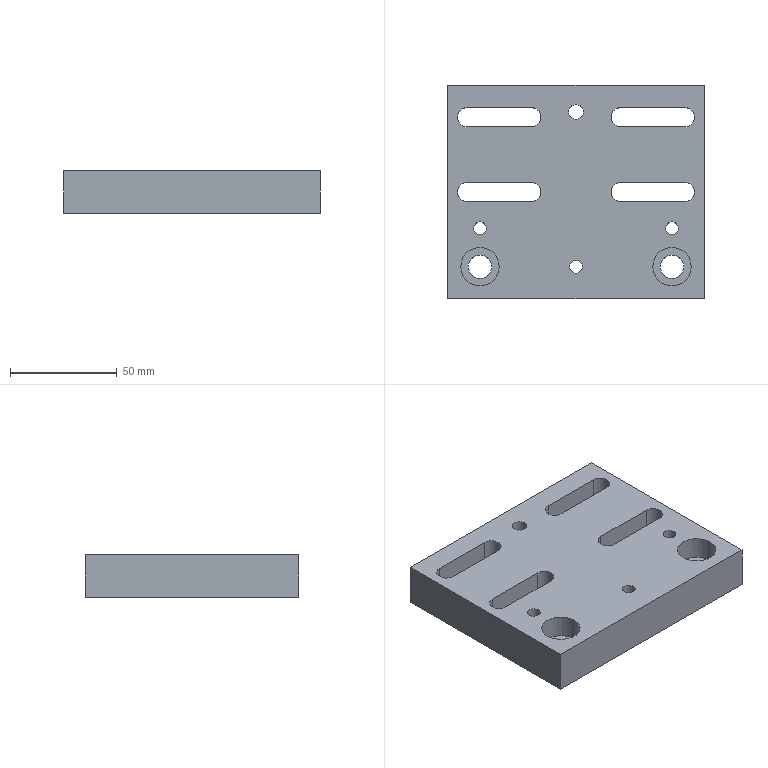Part | NX | 1 solid | 32 faces | box 120 x 100 x 20 mm | volume 203706 mm3 | plane 16 | cylinder 16 | commonest cylinder face diameters 9 x8 6 x3 11 x2 18 x2 6.8 x1
STEP:
#1=CARTESIAN_POINT('',(51.,89.5,0.));
#2=VERTEX_POINT('',#1);
#3=CARTESIAN_POINT('',(51.,89.5,20.));
#4=VERTEX_POINT('',#3);
#5=CARTESIAN_POINT('',(51.,89.5,0.));
#6=DIRECTION('',(0.,0.,1.));
#7=VECTOR('',#6,1000.);
#8=LINE('',#5,#7);
#9=EDGE_CURVE('',#2,#4,#8,.T.);
#10=ORIENTED_EDGE('',*,*,#9,.T.);
#11=CARTESIAN_POINT('',(21.,89.5,20.));
#12=VERTEX_POINT('',#11);
#13=CARTESIAN_POINT('',(21.,89.5,20.));
#14=DIRECTION('',(1.,0.,0.));
#15=VECTOR('',#14,1000.);
#16=LINE('',#13,#15);
#17=EDGE_CURVE('',#12,#4,#16,.T.);
#18=ORIENTED_EDGE('',*,*,#17,.F.);
#19=CARTESIAN_POINT('',(21.,89.5,0.));
#20=VERTEX_POINT('',#19);
#21=CARTESIAN_POINT('',(21.,89.5,0.));
#22=DIRECTION('',(0.,0.,-1.));
#23=VECTOR('',#22,1000.);
#24=LINE('',#21,#23);
#25=EDGE_CURVE('',#12,#20,#24,.T.);
#26=ORIENTED_EDGE('',*,*,#25,.T.);
#27=CARTESIAN_POINT('',(21.,89.5,0.));
#28=DIRECTION('',(1.,0.,0.));
#29=VECTOR('',#28,1000.);
#30=LINE('',#27,#29);
#31=EDGE_CURVE('',#20,#2,#30,.T.);
#32=ORIENTED_EDGE('',*,*,#31,.T.);
#33=EDGE_LOOP('',(#10,#18,#26,#32));
#34=FACE_BOUND('',#33,.T.);
#35=CARTESIAN_POINT('',(21.,89.5,0.));
#36=DIRECTION('',(0.,1.,0.));
#37=DIRECTION('',(0.,0.,1.));
#38=AXIS2_PLACEMENT_3D('',#35,#36,#37);
#39=PLANE('',#38);
#40=ADVANCED_FACE('',(#34),#39,.F.);
#41=CARTESIAN_POINT('',(51.,80.5,20.));
#42=VERTEX_POINT('',#41);
#43=CARTESIAN_POINT('',(51.,80.5,0.));
#44=VERTEX_POINT('',#43);
#45=CARTESIAN_POINT('',(51.,80.5,0.));
#46=DIRECTION('',(0.,0.,-1.));
#47=VECTOR('',#46,1000.);
#48=LINE('',#45,#47);
#49=EDGE_CURVE('',#42,#44,#48,.T.);
#50=ORIENTED_EDGE('',*,*,#49,.T.);
#51=CARTESIAN_POINT('',(21.,80.5,0.));
#52=VERTEX_POINT('',#51);
#53=CARTESIAN_POINT('',(21.,80.5,0.));
#54=DIRECTION('',(1.,0.,0.));
#55=VECTOR('',#54,1000.);
#56=LINE('',#53,#55);
#57=EDGE_CURVE('',#52,#44,#56,.T.);
#58=ORIENTED_EDGE('',*,*,#57,.F.);
#59=CARTESIAN_POINT('',(21.,80.5,20.));
#60=VERTEX_POINT('',#59);
#61=CARTESIAN_POINT('',(21.,80.5,0.));
#62=DIRECTION('',(0.,0.,1.));
#63=VECTOR('',#62,1000.);
#64=LINE('',#61,#63);
#65=EDGE_CURVE('',#52,#60,#64,.T.);
#66=ORIENTED_EDGE('',*,*,#65,.T.);
#67=CARTESIAN_POINT('',(21.,80.5,20.));
#68=DIRECTION('',(1.,0.,0.));
#69=VECTOR('',#68,1000.);
#70=LINE('',#67,#69);
#71=EDGE_CURVE('',#60,#42,#70,.T.);
#72=ORIENTED_EDGE('',*,*,#71,.T.);
#73=EDGE_LOOP('',(#50,#58,#66,#72));
#74=FACE_BOUND('',#73,.T.);
#75=CARTESIAN_POINT('',(21.,80.5,0.));
#76=DIRECTION('',(0.,-1.,0.));
#77=DIRECTION('',(0.,0.,-1.));
#78=AXIS2_PLACEMENT_3D('',#75,#76,#77);
#79=PLANE('',#78);
#80=ADVANCED_FACE('',(#74),#79,.F.);
#81=CARTESIAN_POINT('',(51.,85.,20.));
#82=DIRECTION('',(0.,0.,-1.));
#83=DIRECTION('',(-1.,0.,0.));
#84=AXIS2_PLACEMENT_3D('',#81,#82,#83);
#85=CIRCLE('',#84,4.5);
#86=EDGE_CURVE('',#4,#42,#85,.T.);
#87=ORIENTED_EDGE('',*,*,#86,.F.);
#88=ORIENTED_EDGE('',*,*,#9,.F.);
#89=CARTESIAN_POINT('',(51.,85.,0.));
#90=DIRECTION('',(0.,0.,-1.));
#91=DIRECTION('',(-1.,0.,0.));
#92=AXIS2_PLACEMENT_3D('',#89,#90,#91);
#93=CIRCLE('',#92,4.5);
#94=EDGE_CURVE('',#2,#44,#93,.T.);
#95=ORIENTED_EDGE('',*,*,#94,.T.);
#96=ORIENTED_EDGE('',*,*,#49,.F.);
#97=EDGE_LOOP('',(#87,#88,#95,#96));
#98=FACE_BOUND('',#97,.T.);
#99=CARTESIAN_POINT('',(51.,85.,0.));
#100=DIRECTION('',(0.,0.,-1.));
#101=DIRECTION('',(-1.,0.,0.));
#102=AXIS2_PLACEMENT_3D('',#99,#100,#101);
#103=CYLINDRICAL_SURFACE('',#102,4.5);
#104=ADVANCED_FACE('',(#98),#103,.F.);
#105=CARTESIAN_POINT('',(51.,54.5,0.));
#106=VERTEX_POINT('',#105);
#107=CARTESIAN_POINT('',(51.,54.5,20.));
#108=VERTEX_POINT('',#107);
#109=CARTESIAN_POINT('',(51.,54.5,0.));
#110=DIRECTION('',(0.,0.,1.));
#111=VECTOR('',#110,1000.);
#112=LINE('',#109,#111);
#113=EDGE_CURVE('',#106,#108,#112,.T.);
#114=ORIENTED_EDGE('',*,*,#113,.T.);
#115=CARTESIAN_POINT('',(21.,54.5,20.));
#116=VERTEX_POINT('',#115);
#117=CARTESIAN_POINT('',(21.,54.5,20.));
#118=DIRECTION('',(1.,0.,0.));
#119=VECTOR('',#118,1000.);
#120=LINE('',#117,#119);
#121=EDGE_CURVE('',#116,#108,#120,.T.);
#122=ORIENTED_EDGE('',*,*,#121,.F.);
#123=CARTESIAN_POINT('',(21.,54.5,0.));
#124=VERTEX_POINT('',#123);
#125=CARTESIAN_POINT('',(21.,54.5,0.));
#126=DIRECTION('',(0.,0.,-1.));
#127=VECTOR('',#126,1000.);
#128=LINE('',#125,#127);
#129=EDGE_CURVE('',#116,#124,#128,.T.);
#130=ORIENTED_EDGE('',*,*,#129,.T.);
#131=CARTESIAN_POINT('',(21.,54.5,0.));
#132=DIRECTION('',(1.,0.,0.));
#133=VECTOR('',#132,1000.);
#134=LINE('',#131,#133);
#135=EDGE_CURVE('',#124,#106,#134,.T.);
#136=ORIENTED_EDGE('',*,*,#135,.T.);
#137=EDGE_LOOP('',(#114,#122,#130,#136));
#138=FACE_BOUND('',#137,.T.);
#139=CARTESIAN_POINT('',(21.,54.5,0.));
#140=DIRECTION('',(0.,1.,0.));
#141=DIRECTION('',(0.,0.,1.));
#142=AXIS2_PLACEMENT_3D('',#139,#140,#141);
#143=PLANE('',#142);
#144=ADVANCED_FACE('',(#138),#143,.F.);
#145=CARTESIAN_POINT('',(51.,45.5,20.));
#146=VERTEX_POINT('',#145);
#147=CARTESIAN_POINT('',(51.,45.5,0.));
#148=VERTEX_POINT('',#147);
#149=CARTESIAN_POINT('',(51.,45.5,0.));
#150=DIRECTION('',(0.,0.,-1.));
#151=VECTOR('',#150,1000.);
#152=LINE('',#149,#151);
#153=EDGE_CURVE('',#146,#148,#152,.T.);
#154=ORIENTED_EDGE('',*,*,#153,.T.);
#155=CARTESIAN_POINT('',(21.,45.5,0.));
#156=VERTEX_POINT('',#155);
#157=CARTESIAN_POINT('',(21.,45.5,0.));
#158=DIRECTION('',(1.,0.,0.));
#159=VECTOR('',#158,1000.);
#160=LINE('',#157,#159);
#161=EDGE_CURVE('',#156,#148,#160,.T.);
#162=ORIENTED_EDGE('',*,*,#161,.F.);
#163=CARTESIAN_POINT('',(21.,45.5,20.));
#164=VERTEX_POINT('',#163);
#165=CARTESIAN_POINT('',(21.,45.5,0.));
#166=DIRECTION('',(0.,0.,1.));
#167=VECTOR('',#166,1000.);
#168=LINE('',#165,#167);
#169=EDGE_CURVE('',#156,#164,#168,.T.);
#170=ORIENTED_EDGE('',*,*,#169,.T.);
#171=CARTESIAN_POINT('',(21.,45.5,20.));
#172=DIRECTION('',(1.,0.,0.));
#173=VECTOR('',#172,1000.);
#174=LINE('',#171,#173);
#175=EDGE_CURVE('',#164,#146,#174,.T.);
#176=ORIENTED_EDGE('',*,*,#175,.T.);
#177=EDGE_LOOP('',(#154,#162,#170,#176));
#178=FACE_BOUND('',#177,.T.);
#179=CARTESIAN_POINT('',(21.,45.5,0.));
#180=DIRECTION('',(0.,-1.,0.));
#181=DIRECTION('',(0.,0.,-1.));
#182=AXIS2_PLACEMENT_3D('',#179,#180,#181);
#183=PLANE('',#182);
#184=ADVANCED_FACE('',(#178),#183,.F.);
#185=CARTESIAN_POINT('',(51.,50.,20.));
#186=DIRECTION('',(0.,0.,-1.));
#187=DIRECTION('',(-1.,0.,0.));
#188=AXIS2_PLACEMENT_3D('',#185,#186,#187);
#189=CIRCLE('',#188,4.5);
#190=EDGE_CURVE('',#108,#146,#189,.T.);
#191=ORIENTED_EDGE('',*,*,#190,.F.);
#192=ORIENTED_EDGE('',*,*,#113,.F.);
#193=CARTESIAN_POINT('',(51.,50.,0.));
#194=DIRECTION('',(0.,0.,-1.));
#195=DIRECTION('',(-1.,0.,0.));
#196=AXIS2_PLACEMENT_3D('',#193,#194,#195);
#197=CIRCLE('',#196,4.5);
#198=EDGE_CURVE('',#106,#148,#197,.T.);
#199=ORIENTED_EDGE('',*,*,#198,.T.);
#200=ORIENTED_EDGE('',*,*,#153,.F.);
#201=EDGE_LOOP('',(#191,#192,#199,#200));
#202=FACE_BOUND('',#201,.T.);
#203=CARTESIAN_POINT('',(51.,50.,0.));
#204=DIRECTION('',(0.,0.,-1.));
#205=DIRECTION('',(-1.,0.,0.));
#206=AXIS2_PLACEMENT_3D('',#203,#204,#205);
#207=CYLINDRICAL_SURFACE('',#206,4.5);
#208=ADVANCED_FACE('',(#202),#207,.F.);
#209=CARTESIAN_POINT('',(-21.,89.5,0.));
#210=VERTEX_POINT('',#209);
#211=CARTESIAN_POINT('',(-21.,89.5,20.));
#212=VERTEX_POINT('',#211);
#213=CARTESIAN_POINT('',(-21.,89.5,0.));
#214=DIRECTION('',(0.,0.,1.));
#215=VECTOR('',#214,1000.);
#216=LINE('',#213,#215);
#217=EDGE_CURVE('',#210,#212,#216,.T.);
#218=ORIENTED_EDGE('',*,*,#217,.T.);
#219=CARTESIAN_POINT('',(-51.,89.5,20.));
#220=VERTEX_POINT('',#219);
#221=CARTESIAN_POINT('',(0.,89.5,20.));
#222=DIRECTION('',(1.,0.,0.));
#223=VECTOR('',#222,1000.);
#224=LINE('',#221,#223);
#225=EDGE_CURVE('',#220,#212,#224,.T.);
#226=ORIENTED_EDGE('',*,*,#225,.F.);
#227=CARTESIAN_POINT('',(-51.,89.5,0.));
#228=VERTEX_POINT('',#227);
#229=CARTESIAN_POINT('',(-51.,89.5,0.));
#230=DIRECTION('',(0.,0.,-1.));
#231=VECTOR('',#230,1000.);
#232=LINE('',#229,#231);
#233=EDGE_CURVE('',#220,#228,#232,.T.);
#234=ORIENTED_EDGE('',*,*,#233,.T.);
#235=CARTESIAN_POINT('',(21.,89.5,0.));
#236=DIRECTION('',(1.,0.,0.));
#237=VECTOR('',#236,1000.);
#238=LINE('',#235,#237);
#239=EDGE_CURVE('',#228,#210,#238,.T.);
#240=ORIENTED_EDGE('',*,*,#239,.T.);
#241=EDGE_LOOP('',(#218,#226,#234,#240));
#242=FACE_BOUND('',#241,.T.);
#243=CARTESIAN_POINT('',(21.,89.5,0.));
#244=DIRECTION('',(0.,1.,0.));
#245=DIRECTION('',(0.,0.,1.));
#246=AXIS2_PLACEMENT_3D('',#243,#244,#245);
#247=PLANE('',#246);
#248=ADVANCED_FACE('',(#242),#247,.F.);
#249=CARTESIAN_POINT('',(-21.,80.5,20.));
#250=VERTEX_POINT('',#249);
#251=CARTESIAN_POINT('',(-21.,80.5,0.));
#252=VERTEX_POINT('',#251);
#253=CARTESIAN_POINT('',(-21.,80.5,0.));
#254=DIRECTION('',(0.,0.,-1.));
#255=VECTOR('',#254,1000.);
#256=LINE('',#253,#255);
#257=EDGE_CURVE('',#250,#252,#256,.T.);
#258=ORIENTED_EDGE('',*,*,#257,.T.);
#259=CARTESIAN_POINT('',(-51.,80.5,0.));
#260=VERTEX_POINT('',#259);
#261=CARTESIAN_POINT('',(0.,80.5,0.));
#262=DIRECTION('',(1.,0.,0.));
#263=VECTOR('',#262,1000.);
#264=LINE('',#261,#263);
#265=EDGE_CURVE('',#260,#252,#264,.T.);
#266=ORIENTED_EDGE('',*,*,#265,.F.);
#267=CARTESIAN_POINT('',(-51.,80.5,20.));
#268=VERTEX_POINT('',#267);
#269=CARTESIAN_POINT('',(-51.,80.5,0.));
#270=DIRECTION('',(0.,0.,1.));
#271=VECTOR('',#270,1000.);
#272=LINE('',#269,#271);
#273=EDGE_CURVE('',#260,#268,#272,.T.);
#274=ORIENTED_EDGE('',*,*,#273,.T.);
#275=CARTESIAN_POINT('',(21.,80.5,20.));
#276=DIRECTION('',(1.,0.,0.));
#277=VECTOR('',#276,1000.);
#278=LINE('',#275,#277);
#279=EDGE_CURVE('',#268,#250,#278,.T.);
#280=ORIENTED_EDGE('',*,*,#279,.T.);
#281=EDGE_LOOP('',(#258,#266,#274,#280));
#282=FACE_BOUND('',#281,.T.);
#283=CARTESIAN_POINT('',(21.,80.5,0.));
#284=DIRECTION('',(0.,-1.,0.));
#285=DIRECTION('',(0.,0.,-1.));
#286=AXIS2_PLACEMENT_3D('',#283,#284,#285);
#287=PLANE('',#286);
#288=ADVANCED_FACE('',(#282),#287,.F.);
#289=CARTESIAN_POINT('',(-21.,85.,20.));
#290=DIRECTION('',(0.,0.,-1.));
#291=DIRECTION('',(-1.,0.,0.));
#292=AXIS2_PLACEMENT_3D('',#289,#290,#291);
#293=CIRCLE('',#292,4.5);
#294=EDGE_CURVE('',#212,#250,#293,.T.);
#295=ORIENTED_EDGE('',*,*,#294,.F.);
#296=ORIENTED_EDGE('',*,*,#217,.F.);
#297=CARTESIAN_POINT('',(-21.,85.,0.));
#298=DIRECTION('',(0.,0.,-1.));
#299=DIRECTION('',(-1.,0.,0.));
#300=AXIS2_PLACEMENT_3D('',#297,#298,#299);
#301=CIRCLE('',#300,4.5);
#302=EDGE_CURVE('',#210,#252,#301,.T.);
#303=ORIENTED_EDGE('',*,*,#302,.T.);
#304=ORIENTED_EDGE('',*,*,#257,.F.);
#305=EDGE_LOOP('',(#295,#296,#303,#304));
#306=FACE_BOUND('',#305,.T.);
#307=CARTESIAN_POINT('',(-21.,85.,0.));
#308=DIRECTION('',(0.,0.,-1.));
#309=DIRECTION('',(-1.,0.,0.));
#310=AXIS2_PLACEMENT_3D('',#307,#308,#309);
#311=CYLINDRICAL_SURFACE('',#310,4.5);
#312=ADVANCED_FACE('',(#306),#311,.F.);
#313=CARTESIAN_POINT('',(-21.,54.5,0.));
#314=VERTEX_POINT('',#313);
#315=CARTESIAN_POINT('',(-21.,54.5,20.));
#316=VERTEX_POINT('',#315);
#317=CARTESIAN_POINT('',(-21.,54.5,0.));
#318=DIRECTION('',(0.,0.,1.));
#319=VECTOR('',#318,1000.);
#320=LINE('',#317,#319);
#321=EDGE_CURVE('',#314,#316,#320,.T.);
#322=ORIENTED_EDGE('',*,*,#321,.T.);
#323=CARTESIAN_POINT('',(-51.,54.5,20.));
#324=VERTEX_POINT('',#323);
#325=CARTESIAN_POINT('',(0.,54.5,20.));
#326=DIRECTION('',(1.,0.,0.));
#327=VECTOR('',#326,1000.);
#328=LINE('',#325,#327);
#329=EDGE_CURVE('',#324,#316,#328,.T.);
#330=ORIENTED_EDGE('',*,*,#329,.F.);
#331=CARTESIAN_POINT('',(-51.,54.5,0.));
#332=VERTEX_POINT('',#331);
#333=CARTESIAN_POINT('',(-51.,54.5,0.));
#334=DIRECTION('',(0.,0.,-1.));
#335=VECTOR('',#334,1000.);
#336=LINE('',#333,#335);
#337=EDGE_CURVE('',#324,#332,#336,.T.);
#338=ORIENTED_EDGE('',*,*,#337,.T.);
#339=CARTESIAN_POINT('',(21.,54.5,0.));
#340=DIRECTION('',(1.,0.,0.));
#341=VECTOR('',#340,1000.);
#342=LINE('',#339,#341);
#343=EDGE_CURVE('',#332,#314,#342,.T.);
#344=ORIENTED_EDGE('',*,*,#343,.T.);
#345=EDGE_LOOP('',(#322,#330,#338,#344));
#346=FACE_BOUND('',#345,.T.);
#347=CARTESIAN_POINT('',(21.,54.5,0.));
#348=DIRECTION('',(0.,1.,0.));
#349=DIRECTION('',(0.,0.,1.));
#350=AXIS2_PLACEMENT_3D('',#347,#348,#349);
#351=PLANE('',#350);
#352=ADVANCED_FACE('',(#346),#351,.F.);
#353=CARTESIAN_POINT('',(-21.,45.5,20.));
#354=VERTEX_POINT('',#353);
#355=CARTESIAN_POINT('',(-21.,45.5,0.));
#356=VERTEX_POINT('',#355);
#357=CARTESIAN_POINT('',(-21.,45.5,0.));
#358=DIRECTION('',(0.,0.,-1.));
#359=VECTOR('',#358,1000.);
#360=LINE('',#357,#359);
#361=EDGE_CURVE('',#354,#356,#360,.T.);
#362=ORIENTED_EDGE('',*,*,#361,.T.);
#363=CARTESIAN_POINT('',(-51.,45.5,0.));
#364=VERTEX_POINT('',#363);
#365=CARTESIAN_POINT('',(0.,45.5,0.));
#366=DIRECTION('',(1.,0.,0.));
#367=VECTOR('',#366,1000.);
#368=LINE('',#365,#367);
#369=EDGE_CURVE('',#364,#356,#368,.T.);
#370=ORIENTED_EDGE('',*,*,#369,.F.);
#371=CARTESIAN_POINT('',(-51.,45.5,20.));
#372=VERTEX_POINT('',#371);
#373=CARTESIAN_POINT('',(-51.,45.5,0.));
#374=DIRECTION('',(0.,0.,1.));
#375=VECTOR('',#374,1000.);
#376=LINE('',#373,#375);
#377=EDGE_CURVE('',#364,#372,#376,.T.);
#378=ORIENTED_EDGE('',*,*,#377,.T.);
#379=CARTESIAN_POINT('',(21.,45.5,20.));
#380=DIRECTION('',(1.,0.,0.));
#381=VECTOR('',#380,1000.);
#382=LINE('',#379,#381);
#383=EDGE_CURVE('',#372,#354,#382,.T.);
#384=ORIENTED_EDGE('',*,*,#383,.T.);
#385=EDGE_LOOP('',(#362,#370,#378,#384));
#386=FACE_BOUND('',#385,.T.);
#387=CARTESIAN_POINT('',(21.,45.5,0.));
#388=DIRECTION('',(0.,-1.,0.));
#389=DIRECTION('',(0.,0.,-1.));
#390=AXIS2_PLACEMENT_3D('',#387,#388,#389);
#391=PLANE('',#390);
#392=ADVANCED_FACE('',(#386),#391,.F.);
#393=CARTESIAN_POINT('',(-21.,50.,20.));
#394=DIRECTION('',(0.,0.,-1.));
#395=DIRECTION('',(-1.,0.,0.));
#396=AXIS2_PLACEMENT_3D('',#393,#394,#395);
#397=CIRCLE('',#396,4.5);
#398=EDGE_CURVE('',#316,#354,#397,.T.);
#399=ORIENTED_EDGE('',*,*,#398,.F.);
#400=ORIENTED_EDGE('',*,*,#321,.F.);
#401=CARTESIAN_POINT('',(-21.,50.,0.));
#402=DIRECTION('',(0.,0.,-1.));
#403=DIRECTION('',(-1.,0.,0.));
#404=AXIS2_PLACEMENT_3D('',#401,#402,#403);
#405=CIRCLE('',#404,4.5);
#406=EDGE_CURVE('',#314,#356,#405,.T.);
#407=ORIENTED_EDGE('',*,*,#406,.T.);
#408=ORIENTED_EDGE('',*,*,#361,.F.);
#409=EDGE_LOOP('',(#399,#400,#407,#408));
#410=FACE_BOUND('',#409,.T.);
#411=CARTESIAN_POINT('',(-21.,50.,0.));
#412=DIRECTION('',(0.,0.,-1.));
#413=DIRECTION('',(-1.,0.,0.));
#414=AXIS2_PLACEMENT_3D('',#411,#412,#413);
#415=CYLINDRICAL_SURFACE('',#414,4.5);
#416=ADVANCED_FACE('',(#410),#415,.F.);
#417=CARTESIAN_POINT('',(54.,15.,9.4));
#418=VERTEX_POINT('',#417);
#419=CARTESIAN_POINT('',(45.,15.,9.4));
#420=DIRECTION('',(0.,0.,1.));
#421=DIRECTION('',(1.,0.,0.));
#422=AXIS2_PLACEMENT_3D('',#419,#420,#421);
#423=CIRCLE('',#422,9.);
#424=EDGE_CURVE('',#418,#418,#423,.T.);
#425=ORIENTED_EDGE('',*,*,#424,.T.);
#426=EDGE_LOOP('',(#425));
#427=FACE_BOUND('',#426,.T.);
#428=CARTESIAN_POINT('',(50.5,15.,9.4));
#429=VERTEX_POINT('',#428);
#430=CARTESIAN_POINT('',(45.,15.,9.4));
#431=DIRECTION('',(0.,0.,1.));
#432=DIRECTION('',(1.,0.,0.));
#433=AXIS2_PLACEMENT_3D('',#430,#431,#432);
#434=CIRCLE('',#433,5.5);
#435=EDGE_CURVE('',#429,#429,#434,.T.);
#436=ORIENTED_EDGE('',*,*,#435,.F.);
#437=EDGE_LOOP('',(#436));
#438=FACE_BOUND('',#437,.T.);
#439=CARTESIAN_POINT('',(50.5,15.,9.4));
#440=DIRECTION('',(0.,0.,-1.));
#441=DIRECTION('',(-1.,0.,0.));
#442=AXIS2_PLACEMENT_3D('',#439,#440,#441);
#443=PLANE('',#442);
#444=ADVANCED_FACE('',(#427,#438),#443,.F.);
#445=CARTESIAN_POINT('',(-54.,15.,9.4));
#446=VERTEX_POINT('',#445);
#447=CARTESIAN_POINT('',(-45.,15.,9.4));
#448=DIRECTION('',(0.,0.,1.));
#449=DIRECTION('',(-1.,0.,0.));
#450=AXIS2_PLACEMENT_3D('',#447,#448,#449);
#451=CIRCLE('',#450,9.);
#452=EDGE_CURVE('',#446,#446,#451,.T.);
#453=ORIENTED_EDGE('',*,*,#452,.T.);
#454=EDGE_LOOP('',(#453));
#455=FACE_BOUND('',#454,.T.);
#456=CARTESIAN_POINT('',(-50.5,15.,9.4));
#457=VERTEX_POINT('',#456);
#458=CARTESIAN_POINT('',(-45.,15.,9.4));
#459=DIRECTION('',(0.,0.,1.));
#460=DIRECTION('',(-1.,0.,0.));
#461=AXIS2_PLACEMENT_3D('',#458,#459,#460);
#462=CIRCLE('',#461,5.5);
#463=EDGE_CURVE('',#457,#457,#462,.T.);
#464=ORIENTED_EDGE('',*,*,#463,.F.);
#465=EDGE_LOOP('',(#464));
#466=FACE_BOUND('',#465,.T.);
#467=CARTESIAN_POINT('',(50.5,15.,9.4));
#468=DIRECTION('',(0.,0.,-1.));
#469=DIRECTION('',(-1.,0.,0.));
#470=AXIS2_PLACEMENT_3D('',#467,#468,#469);
#471=PLANE('',#470);
#472=ADVANCED_FACE('',(#455,#466),#471,.F.);
#473=CARTESIAN_POINT('',(-60.,100.,0.));
#474=VERTEX_POINT('',#473);
#475=CARTESIAN_POINT('',(-60.,0.,0.));
#476=VERTEX_POINT('',#475);
#477=CARTESIAN_POINT('',(-60.,0.,0.));
#478=DIRECTION('',(0.,-1.,0.));
#479=VECTOR('',#478,1000.);
#480=LINE('',#477,#479);
#481=EDGE_CURVE('',#474,#476,#480,.T.);
#482=ORIENTED_EDGE('',*,*,#481,.F.);
#483=CARTESIAN_POINT('',(60.,100.,0.));
#484=VERTEX_POINT('',#483);
#485=CARTESIAN_POINT('',(-60.,100.,0.));
#486=DIRECTION('',(-1.,0.,0.));
#487=VECTOR('',#486,1000.);
#488=LINE('',#485,#487);
#489=EDGE_CURVE('',#484,#474,#488,.T.);
#490=ORIENTED_EDGE('',*,*,#489,.F.);
#491=CARTESIAN_POINT('',(60.,0.,0.));
#492=VERTEX_POINT('',#491);
#493=CARTESIAN_POINT('',(60.,0.,0.));
#494=DIRECTION('',(0.,1.,0.));
#495=VECTOR('',#494,1000.);
#496=LINE('',#493,#495);
#497=EDGE_CURVE('',#492,#484,#496,.T.);
#498=ORIENTED_EDGE('',*,*,#497,.F.);
#499=CARTESIAN_POINT('',(-60.,0.,0.));
#500=DIRECTION('',(1.,0.,0.));
#501=VECTOR('',#500,1000.);
#502=LINE('',#499,#501);
#503=EDGE_CURVE('',#476,#492,#502,.T.);
#504=ORIENTED_EDGE('',*,*,#503,.F.);
#505=EDGE_LOOP('',(#482,#490,#498,#504));
#506=FACE_BOUND('',#505,.T.);
#507=CARTESIAN_POINT('',(-39.5,15.,0.));
#508=VERTEX_POINT('',#507);
#509=CARTESIAN_POINT('',(-45.,15.,0.));
#510=DIRECTION('',(0.,0.,1.));
#511=DIRECTION('',(1.,0.,0.));
#512=AXIS2_PLACEMENT_3D('',#509,#510,#511);
#513=CIRCLE('',#512,5.5);
#514=EDGE_CURVE('',#508,#508,#513,.T.);
#515=ORIENTED_EDGE('',*,*,#514,.T.);
#516=EDGE_LOOP('',(#515));
#517=FACE_BOUND('',#516,.T.);
#518=CARTESIAN_POINT('',(50.5,15.,0.));
#519=VERTEX_POINT('',#518);
#520=CARTESIAN_POINT('',(45.,15.,0.));
#521=DIRECTION('',(0.,0.,1.));
#522=DIRECTION('',(1.,0.,0.));
#523=AXIS2_PLACEMENT_3D('',#520,#521,#522);
#524=CIRCLE('',#523,5.5);
#525=EDGE_CURVE('',#519,#519,#524,.T.);
#526=ORIENTED_EDGE('',*,*,#525,.T.);
#527=EDGE_LOOP('',(#526));
#528=FACE_BOUND('',#527,.T.);
#529=CARTESIAN_POINT('',(42.,33.,0.));
#530=VERTEX_POINT('',#529);
#531=CARTESIAN_POINT('',(45.,33.,0.));
#532=DIRECTION('',(0.,0.,-1.));
#533=DIRECTION('',(-1.,0.,0.));
#534=AXIS2_PLACEMENT_3D('',#531,#532,#533);
#535=CIRCLE('',#534,3.);
#536=EDGE_CURVE('',#530,#530,#535,.T.);
#537=ORIENTED_EDGE('',*,*,#536,.F.);
#538=EDGE_LOOP('',(#537));
#539=FACE_BOUND('',#538,.T.);
#540=CARTESIAN_POINT('',(-48.,33.,0.));
#541=VERTEX_POINT('',#540);
#542=CARTESIAN_POINT('',(-45.,33.,0.));
#543=DIRECTION('',(0.,0.,-1.));
#544=DIRECTION('',(-1.,0.,0.));
#545=AXIS2_PLACEMENT_3D('',#542,#543,#544);
#546=CIRCLE('',#545,3.);
#547=EDGE_CURVE('',#541,#541,#546,.T.);
#548=ORIENTED_EDGE('',*,*,#547,.F.);
#549=EDGE_LOOP('',(#548));
#550=FACE_BOUND('',#549,.T.);
#551=CARTESIAN_POINT('',(-3.,15.,0.));
#552=VERTEX_POINT('',#551);
#553=CARTESIAN_POINT('',(0.,15.,0.));
#554=DIRECTION('',(0.,0.,-1.));
#555=DIRECTION('',(-1.,0.,0.));
#556=AXIS2_PLACEMENT_3D('',#553,#554,#555);
#557=CIRCLE('',#556,3.);
#558=EDGE_CURVE('',#552,#552,#557,.T.);
#559=ORIENTED_EDGE('',*,*,#558,.F.);
#560=EDGE_LOOP('',(#559));
#561=FACE_BOUND('',#560,.T.);
#562=ORIENTED_EDGE('',*,*,#406,.F.);
#563=ORIENTED_EDGE('',*,*,#343,.F.);
#564=CARTESIAN_POINT('',(-51.,50.,0.));
#565=DIRECTION('',(0.,0.,-1.));
#566=DIRECTION('',(-1.,0.,0.));
#567=AXIS2_PLACEMENT_3D('',#564,#565,#566);
#568=CIRCLE('',#567,4.5);
#569=EDGE_CURVE('',#364,#332,#568,.T.);
#570=ORIENTED_EDGE('',*,*,#569,.F.);
#571=ORIENTED_EDGE('',*,*,#369,.T.);
#572=EDGE_LOOP('',(#562,#563,#570,#571));
#573=FACE_BOUND('',#572,.T.);
#574=ORIENTED_EDGE('',*,*,#302,.F.);
#575=ORIENTED_EDGE('',*,*,#239,.F.);
#576=CARTESIAN_POINT('',(-51.,85.,0.));
#577=DIRECTION('',(0.,0.,-1.));
#578=DIRECTION('',(-1.,0.,0.));
#579=AXIS2_PLACEMENT_3D('',#576,#577,#578);
#580=CIRCLE('',#579,4.5);
#581=EDGE_CURVE('',#260,#228,#580,.T.);
#582=ORIENTED_EDGE('',*,*,#581,.F.);
#583=ORIENTED_EDGE('',*,*,#265,.T.);
#584=EDGE_LOOP('',(#574,#575,#582,#583));
#585=FACE_BOUND('',#584,.T.);
#586=ORIENTED_EDGE('',*,*,#198,.F.);
#587=ORIENTED_EDGE('',*,*,#135,.F.);
#588=CARTESIAN_POINT('',(21.,50.,0.));
#589=DIRECTION('',(0.,0.,-1.));
#590=DIRECTION('',(-1.,0.,0.));
#591=AXIS2_PLACEMENT_3D('',#588,#589,#590);
#592=CIRCLE('',#591,4.5);
#593=EDGE_CURVE('',#156,#124,#592,.T.);
#594=ORIENTED_EDGE('',*,*,#593,.F.);
#595=ORIENTED_EDGE('',*,*,#161,.T.);
#596=EDGE_LOOP('',(#586,#587,#594,#595));
#597=FACE_BOUND('',#596,.T.);
#598=ORIENTED_EDGE('',*,*,#57,.T.);
#599=ORIENTED_EDGE('',*,*,#94,.F.);
#600=ORIENTED_EDGE('',*,*,#31,.F.);
#601=CARTESIAN_POINT('',(21.,85.,0.));
#602=DIRECTION('',(0.,0.,-1.));
#603=DIRECTION('',(-1.,0.,0.));
#604=AXIS2_PLACEMENT_3D('',#601,#602,#603);
#605=CIRCLE('',#604,4.5);
#606=EDGE_CURVE('',#52,#20,#605,.T.);
#607=ORIENTED_EDGE('',*,*,#606,.F.);
#608=EDGE_LOOP('',(#598,#599,#600,#607));
#609=FACE_BOUND('',#608,.T.);
#610=CARTESIAN_POINT('',(-3.4,87.5,0.));
#611=VERTEX_POINT('',#610);
#612=CARTESIAN_POINT('',(0.,87.5,0.));
#613=DIRECTION('',(0.,0.,-1.));
#614=DIRECTION('',(-1.,0.,0.));
#615=AXIS2_PLACEMENT_3D('',#612,#613,#614);
#616=CIRCLE('',#615,3.4);
#617=EDGE_CURVE('',#611,#611,#616,.T.);
#618=ORIENTED_EDGE('',*,*,#617,.F.);
#619=EDGE_LOOP('',(#618));
#620=FACE_BOUND('',#619,.T.);
#621=CARTESIAN_POINT('',(0.,0.,0.));
#622=DIRECTION('',(0.,0.,-1.));
#623=DIRECTION('',(-1.,0.,0.));
#624=AXIS2_PLACEMENT_3D('',#621,#622,#623);
#625=PLANE('',#624);
#626=ADVANCED_FACE('',(#506,#517,#528,#539,#550,#561,#573,#585,#597,#609,#620),#625,.T.);
#627=ORIENTED_EDGE('',*,*,#489,.T.);
#628=CARTESIAN_POINT('',(-60.,100.,20.));
#629=VERTEX_POINT('',#628);
#630=CARTESIAN_POINT('',(-60.,100.,20.));
#631=DIRECTION('',(0.,0.,-1.));
#632=VECTOR('',#631,1000.);
#633=LINE('',#630,#632);
#634=EDGE_CURVE('',#629,#474,#633,.T.);
#635=ORIENTED_EDGE('',*,*,#634,.F.);
#636=CARTESIAN_POINT('',(60.,100.,20.));
#637=VERTEX_POINT('',#636);
#638=CARTESIAN_POINT('',(-60.,100.,20.));
#639=DIRECTION('',(-1.,0.,0.));
#640=VECTOR('',#639,1000.);
#641=LINE('',#638,#640);
#642=EDGE_CURVE('',#637,#629,#641,.T.);
#643=ORIENTED_EDGE('',*,*,#642,.F.);
#644=CARTESIAN_POINT('',(60.,100.,20.));
#645=DIRECTION('',(0.,0.,-1.));
#646=VECTOR('',#645,1000.);
#647=LINE('',#644,#646);
#648=EDGE_CURVE('',#637,#484,#647,.T.);
#649=ORIENTED_EDGE('',*,*,#648,.T.);
#650=EDGE_LOOP('',(#627,#635,#643,#649));
#651=FACE_BOUND('',#650,.T.);
#652=CARTESIAN_POINT('',(-60.,100.,20.));
#653=DIRECTION('',(0.,-1.,0.));
#654=DIRECTION('',(0.,0.,-1.));
#655=AXIS2_PLACEMENT_3D('',#652,#653,#654);
#656=PLANE('',#655);
#657=ADVANCED_FACE('',(#651),#656,.F.);
#658=ORIENTED_EDGE('',*,*,#497,.T.);
#659=ORIENTED_EDGE('',*,*,#648,.F.);
#660=CARTESIAN_POINT('',(60.,0.,20.));
#661=VERTEX_POINT('',#660);
#662=CARTESIAN_POINT('',(60.,0.,20.));
#663=DIRECTION('',(0.,1.,0.));
#664=VECTOR('',#663,1000.);
#665=LINE('',#662,#664);
#666=EDGE_CURVE('',#661,#637,#665,.T.);
#667=ORIENTED_EDGE('',*,*,#666,.F.);
#668=CARTESIAN_POINT('',(60.,0.,20.));
#669=DIRECTION('',(0.,0.,-1.));
#670=VECTOR('',#669,1000.);
#671=LINE('',#668,#670);
#672=EDGE_CURVE('',#661,#492,#671,.T.);
#673=ORIENTED_EDGE('',*,*,#672,.T.);
#674=EDGE_LOOP('',(#658,#659,#667,#673));
#675=FACE_BOUND('',#674,.T.);
#676=CARTESIAN_POINT('',(60.,0.,20.));
#677=DIRECTION('',(-1.,0.,0.));
#678=DIRECTION('',(0.,0.,1.));
#679=AXIS2_PLACEMENT_3D('',#676,#677,#678);
#680=PLANE('',#679);
#681=ADVANCED_FACE('',(#675),#680,.F.);
#682=ORIENTED_EDGE('',*,*,#503,.T.);
#683=ORIENTED_EDGE('',*,*,#672,.F.);
#684=CARTESIAN_POINT('',(-60.,0.,20.));
#685=VERTEX_POINT('',#684);
#686=CARTESIAN_POINT('',(-60.,0.,20.));
#687=DIRECTION('',(1.,0.,0.));
#688=VECTOR('',#687,1000.);
#689=LINE('',#686,#688);
#690=EDGE_CURVE('',#685,#661,#689,.T.);
#691=ORIENTED_EDGE('',*,*,#690,.F.);
#692=CARTESIAN_POINT('',(-60.,0.,20.));
#693=DIRECTION('',(0.,0.,-1.));
#694=VECTOR('',#693,1000.);
#695=LINE('',#692,#694);
#696=EDGE_CURVE('',#685,#476,#695,.T.);
#697=ORIENTED_EDGE('',*,*,#696,.T.);
#698=EDGE_LOOP('',(#682,#683,#691,#697));
#699=FACE_BOUND('',#698,.T.);
#700=CARTESIAN_POINT('',(-60.,0.,20.));
#701=DIRECTION('',(0.,1.,0.));
#702=DIRECTION('',(0.,0.,1.));
#703=AXIS2_PLACEMENT_3D('',#700,#701,#702);
#704=PLANE('',#703);
#705=ADVANCED_FACE('',(#699),#704,.F.);
#706=ORIENTED_EDGE('',*,*,#481,.T.);
#707=ORIENTED_EDGE('',*,*,#696,.F.);
#708=CARTESIAN_POINT('',(-60.,0.,20.));
#709=DIRECTION('',(0.,-1.,0.));
#710=VECTOR('',#709,1000.);
#711=LINE('',#708,#710);
#712=EDGE_CURVE('',#629,#685,#711,.T.);
#713=ORIENTED_EDGE('',*,*,#712,.F.);
#714=ORIENTED_EDGE('',*,*,#634,.T.);
#715=EDGE_LOOP('',(#706,#707,#713,#714));
#716=FACE_BOUND('',#715,.T.);
#717=CARTESIAN_POINT('',(-60.,0.,20.));
#718=DIRECTION('',(1.,0.,0.));
#719=DIRECTION('',(0.,0.,-1.));
#720=AXIS2_PLACEMENT_3D('',#717,#718,#719);
#721=PLANE('',#720);
#722=ADVANCED_FACE('',(#716),#721,.F.);
#723=ORIENTED_EDGE('',*,*,#175,.F.);
#724=CARTESIAN_POINT('',(21.,50.,20.));
#725=DIRECTION('',(0.,0.,-1.));
#726=DIRECTION('',(-1.,0.,0.));
#727=AXIS2_PLACEMENT_3D('',#724,#725,#726);
#728=CIRCLE('',#727,4.5);
#729=EDGE_CURVE('',#164,#116,#728,.T.);
#730=ORIENTED_EDGE('',*,*,#729,.T.);
#731=ORIENTED_EDGE('',*,*,#121,.T.);
#732=ORIENTED_EDGE('',*,*,#190,.T.);
#733=EDGE_LOOP('',(#723,#730,#731,#732));
#734=FACE_BOUND('',#733,.T.);
#735=ORIENTED_EDGE('',*,*,#294,.T.);
#736=ORIENTED_EDGE('',*,*,#279,.F.);
#737=CARTESIAN_POINT('',(-51.,85.,20.));
#738=DIRECTION('',(0.,0.,-1.));
#739=DIRECTION('',(-1.,0.,0.));
#740=AXIS2_PLACEMENT_3D('',#737,#738,#739);
#741=CIRCLE('',#740,4.5);
#742=EDGE_CURVE('',#268,#220,#741,.T.);
#743=ORIENTED_EDGE('',*,*,#742,.T.);
#744=ORIENTED_EDGE('',*,*,#225,.T.);
#745=EDGE_LOOP('',(#735,#736,#743,#744));
#746=FACE_BOUND('',#745,.T.);
#747=ORIENTED_EDGE('',*,*,#329,.T.);
#748=ORIENTED_EDGE('',*,*,#398,.T.);
#749=ORIENTED_EDGE('',*,*,#383,.F.);
#750=CARTESIAN_POINT('',(-51.,50.,20.));
#751=DIRECTION('',(0.,0.,-1.));
#752=DIRECTION('',(-1.,0.,0.));
#753=AXIS2_PLACEMENT_3D('',#750,#751,#752);
#754=CIRCLE('',#753,4.5);
#755=EDGE_CURVE('',#372,#324,#754,.T.);
#756=ORIENTED_EDGE('',*,*,#755,.T.);
#757=EDGE_LOOP('',(#747,#748,#749,#756));
#758=FACE_BOUND('',#757,.T.);
#759=CARTESIAN_POINT('',(-3.,15.,20.));
#760=VERTEX_POINT('',#759);
#761=CARTESIAN_POINT('',(0.,15.,20.));
#762=DIRECTION('',(0.,0.,-1.));
#763=DIRECTION('',(-1.,0.,0.));
#764=AXIS2_PLACEMENT_3D('',#761,#762,#763);
#765=CIRCLE('',#764,3.);
#766=EDGE_CURVE('',#760,#760,#765,.T.);
#767=ORIENTED_EDGE('',*,*,#766,.T.);
#768=EDGE_LOOP('',(#767));
#769=FACE_BOUND('',#768,.T.);
#770=CARTESIAN_POINT('',(-48.,33.,20.));
#771=VERTEX_POINT('',#770);
#772=CARTESIAN_POINT('',(-45.,33.,20.));
#773=DIRECTION('',(0.,0.,-1.));
#774=DIRECTION('',(-1.,0.,0.));
#775=AXIS2_PLACEMENT_3D('',#772,#773,#774);
#776=CIRCLE('',#775,3.);
#777=EDGE_CURVE('',#771,#771,#776,.T.);
#778=ORIENTED_EDGE('',*,*,#777,.T.);
#779=EDGE_LOOP('',(#778));
#780=FACE_BOUND('',#779,.T.);
#781=CARTESIAN_POINT('',(42.,33.,20.));
#782=VERTEX_POINT('',#781);
#783=CARTESIAN_POINT('',(45.,33.,20.));
#784=DIRECTION('',(0.,0.,-1.));
#785=DIRECTION('',(-1.,0.,0.));
#786=AXIS2_PLACEMENT_3D('',#783,#784,#785);
#787=CIRCLE('',#786,3.);
#788=EDGE_CURVE('',#782,#782,#787,.T.);
#789=ORIENTED_EDGE('',*,*,#788,.T.);
#790=EDGE_LOOP('',(#789));
#791=FACE_BOUND('',#790,.T.);
#792=CARTESIAN_POINT('',(54.,15.,20.));
#793=VERTEX_POINT('',#792);
#794=CARTESIAN_POINT('',(45.,15.,20.));
#795=DIRECTION('',(0.,0.,1.));
#796=DIRECTION('',(1.,0.,0.));
#797=AXIS2_PLACEMENT_3D('',#794,#795,#796);
#798=CIRCLE('',#797,9.);
#799=EDGE_CURVE('',#793,#793,#798,.T.);
#800=ORIENTED_EDGE('',*,*,#799,.F.);
#801=EDGE_LOOP('',(#800));
#802=FACE_BOUND('',#801,.T.);
#803=CARTESIAN_POINT('',(-36.,15.,20.));
#804=VERTEX_POINT('',#803);
#805=CARTESIAN_POINT('',(-45.,15.,20.));
#806=DIRECTION('',(0.,0.,1.));
#807=DIRECTION('',(1.,0.,0.));
#808=AXIS2_PLACEMENT_3D('',#805,#806,#807);
#809=CIRCLE('',#808,9.);
#810=EDGE_CURVE('',#804,#804,#809,.T.);
#811=ORIENTED_EDGE('',*,*,#810,.F.);
#812=EDGE_LOOP('',(#811));
#813=FACE_BOUND('',#812,.T.);
#814=ORIENTED_EDGE('',*,*,#712,.T.);
#815=ORIENTED_EDGE('',*,*,#690,.T.);
#816=ORIENTED_EDGE('',*,*,#666,.T.);
#817=ORIENTED_EDGE('',*,*,#642,.T.);
#818=EDGE_LOOP('',(#814,#815,#816,#817));
#819=FACE_BOUND('',#818,.T.);
#820=ORIENTED_EDGE('',*,*,#17,.T.);
#821=ORIENTED_EDGE('',*,*,#86,.T.);
#822=ORIENTED_EDGE('',*,*,#71,.F.);
#823=CARTESIAN_POINT('',(21.,85.,20.));
#824=DIRECTION('',(0.,0.,-1.));
#825=DIRECTION('',(-1.,0.,0.));
#826=AXIS2_PLACEMENT_3D('',#823,#824,#825);
#827=CIRCLE('',#826,4.5);
#828=EDGE_CURVE('',#60,#12,#827,.T.);
#829=ORIENTED_EDGE('',*,*,#828,.T.);
#830=EDGE_LOOP('',(#820,#821,#822,#829));
#831=FACE_BOUND('',#830,.T.);
#832=CARTESIAN_POINT('',(-3.4,87.5,20.));
#833=VERTEX_POINT('',#832);
#834=CARTESIAN_POINT('',(0.,87.5,20.));
#835=DIRECTION('',(0.,0.,-1.));
#836=DIRECTION('',(-1.,0.,0.));
#837=AXIS2_PLACEMENT_3D('',#834,#835,#836);
#838=CIRCLE('',#837,3.4);
#839=EDGE_CURVE('',#833,#833,#838,.T.);
#840=ORIENTED_EDGE('',*,*,#839,.T.);
#841=EDGE_LOOP('',(#840));
#842=FACE_BOUND('',#841,.T.);
#843=CARTESIAN_POINT('',(0.,0.,20.));
#844=DIRECTION('',(0.,0.,-1.));
#845=DIRECTION('',(-1.,0.,0.));
#846=AXIS2_PLACEMENT_3D('',#843,#844,#845);
#847=PLANE('',#846);
#848=ADVANCED_FACE('',(#734,#746,#758,#769,#780,#791,#802,#813,#819,#831,#842),#847,.F.);
#849=ORIENTED_EDGE('',*,*,#514,.F.);
#850=EDGE_LOOP('',(#849));
#851=FACE_BOUND('',#850,.T.);
#852=ORIENTED_EDGE('',*,*,#463,.T.);
#853=EDGE_LOOP('',(#852));
#854=FACE_BOUND('',#853,.T.);
#855=CARTESIAN_POINT('',(-45.,15.,20.));
#856=DIRECTION('',(0.,0.,1.));
#857=DIRECTION('',(1.,0.,0.));
#858=AXIS2_PLACEMENT_3D('',#855,#856,#857);
#859=CYLINDRICAL_SURFACE('',#858,5.5);
#860=ADVANCED_FACE('',(#851,#854),#859,.F.);
#861=ORIENTED_EDGE('',*,*,#452,.F.);
#862=EDGE_LOOP('',(#861));
#863=FACE_BOUND('',#862,.T.);
#864=ORIENTED_EDGE('',*,*,#810,.T.);
#865=EDGE_LOOP('',(#864));
#866=FACE_BOUND('',#865,.T.);
#867=CARTESIAN_POINT('',(-45.,15.,20.));
#868=DIRECTION('',(0.,0.,1.));
#869=DIRECTION('',(1.,0.,0.));
#870=AXIS2_PLACEMENT_3D('',#867,#868,#869);
#871=CYLINDRICAL_SURFACE('',#870,9.);
#872=ADVANCED_FACE('',(#863,#866),#871,.F.);
#873=ORIENTED_EDGE('',*,*,#525,.F.);
#874=EDGE_LOOP('',(#873));
#875=FACE_BOUND('',#874,.T.);
#876=ORIENTED_EDGE('',*,*,#435,.T.);
#877=EDGE_LOOP('',(#876));
#878=FACE_BOUND('',#877,.T.);
#879=CARTESIAN_POINT('',(45.,15.,20.));
#880=DIRECTION('',(0.,0.,1.));
#881=DIRECTION('',(1.,0.,0.));
#882=AXIS2_PLACEMENT_3D('',#879,#880,#881);
#883=CYLINDRICAL_SURFACE('',#882,5.5);
#884=ADVANCED_FACE('',(#875,#878),#883,.F.);
#885=ORIENTED_EDGE('',*,*,#424,.F.);
#886=EDGE_LOOP('',(#885));
#887=FACE_BOUND('',#886,.T.);
#888=ORIENTED_EDGE('',*,*,#799,.T.);
#889=EDGE_LOOP('',(#888));
#890=FACE_BOUND('',#889,.T.);
#891=CARTESIAN_POINT('',(45.,15.,20.));
#892=DIRECTION('',(0.,0.,1.));
#893=DIRECTION('',(1.,0.,0.));
#894=AXIS2_PLACEMENT_3D('',#891,#892,#893);
#895=CYLINDRICAL_SURFACE('',#894,9.);
#896=ADVANCED_FACE('',(#887,#890),#895,.F.);
#897=ORIENTED_EDGE('',*,*,#536,.T.);
#898=EDGE_LOOP('',(#897));
#899=FACE_BOUND('',#898,.T.);
#900=ORIENTED_EDGE('',*,*,#788,.F.);
#901=EDGE_LOOP('',(#900));
#902=FACE_BOUND('',#901,.T.);
#903=CARTESIAN_POINT('',(45.,33.,0.));
#904=DIRECTION('',(0.,0.,-1.));
#905=DIRECTION('',(-1.,0.,0.));
#906=AXIS2_PLACEMENT_3D('',#903,#904,#905);
#907=CYLINDRICAL_SURFACE('',#906,3.);
#908=ADVANCED_FACE('',(#899,#902),#907,.F.);
#909=ORIENTED_EDGE('',*,*,#547,.T.);
#910=EDGE_LOOP('',(#909));
#911=FACE_BOUND('',#910,.T.);
#912=ORIENTED_EDGE('',*,*,#777,.F.);
#913=EDGE_LOOP('',(#912));
#914=FACE_BOUND('',#913,.T.);
#915=CARTESIAN_POINT('',(-45.,33.,0.));
#916=DIRECTION('',(0.,0.,-1.));
#917=DIRECTION('',(-1.,0.,0.));
#918=AXIS2_PLACEMENT_3D('',#915,#916,#917);
#919=CYLINDRICAL_SURFACE('',#918,3.);
#920=ADVANCED_FACE('',(#911,#914),#919,.F.);
#921=ORIENTED_EDGE('',*,*,#558,.T.);
#922=EDGE_LOOP('',(#921));
#923=FACE_BOUND('',#922,.T.);
#924=ORIENTED_EDGE('',*,*,#766,.F.);
#925=EDGE_LOOP('',(#924));
#926=FACE_BOUND('',#925,.T.);
#927=CARTESIAN_POINT('',(0.,15.,0.));
#928=DIRECTION('',(0.,0.,-1.));
#929=DIRECTION('',(-1.,0.,0.));
#930=AXIS2_PLACEMENT_3D('',#927,#928,#929);
#931=CYLINDRICAL_SURFACE('',#930,3.);
#932=ADVANCED_FACE('',(#923,#926),#931,.F.);
#933=ORIENTED_EDGE('',*,*,#755,.F.);
#934=ORIENTED_EDGE('',*,*,#377,.F.);
#935=ORIENTED_EDGE('',*,*,#569,.T.);
#936=ORIENTED_EDGE('',*,*,#337,.F.);
#937=EDGE_LOOP('',(#933,#934,#935,#936));
#938=FACE_BOUND('',#937,.T.);
#939=CARTESIAN_POINT('',(-51.,50.,0.));
#940=DIRECTION('',(0.,0.,-1.));
#941=DIRECTION('',(-1.,0.,0.));
#942=AXIS2_PLACEMENT_3D('',#939,#940,#941);
#943=CYLINDRICAL_SURFACE('',#942,4.5);
#944=ADVANCED_FACE('',(#938),#943,.F.);
#945=ORIENTED_EDGE('',*,*,#742,.F.);
#946=ORIENTED_EDGE('',*,*,#273,.F.);
#947=ORIENTED_EDGE('',*,*,#581,.T.);
#948=ORIENTED_EDGE('',*,*,#233,.F.);
#949=EDGE_LOOP('',(#945,#946,#947,#948));
#950=FACE_BOUND('',#949,.T.);
#951=CARTESIAN_POINT('',(-51.,85.,0.));
#952=DIRECTION('',(0.,0.,-1.));
#953=DIRECTION('',(-1.,0.,0.));
#954=AXIS2_PLACEMENT_3D('',#951,#952,#953);
#955=CYLINDRICAL_SURFACE('',#954,4.5);
#956=ADVANCED_FACE('',(#950),#955,.F.);
#957=ORIENTED_EDGE('',*,*,#729,.F.);
#958=ORIENTED_EDGE('',*,*,#169,.F.);
#959=ORIENTED_EDGE('',*,*,#593,.T.);
#960=ORIENTED_EDGE('',*,*,#129,.F.);
#961=EDGE_LOOP('',(#957,#958,#959,#960));
#962=FACE_BOUND('',#961,.T.);
#963=CARTESIAN_POINT('',(21.,50.,0.));
#964=DIRECTION('',(0.,0.,-1.));
#965=DIRECTION('',(-1.,0.,0.));
#966=AXIS2_PLACEMENT_3D('',#963,#964,#965);
#967=CYLINDRICAL_SURFACE('',#966,4.5);
#968=ADVANCED_FACE('',(#962),#967,.F.);
#969=ORIENTED_EDGE('',*,*,#828,.F.);
#970=ORIENTED_EDGE('',*,*,#65,.F.);
#971=ORIENTED_EDGE('',*,*,#606,.T.);
#972=ORIENTED_EDGE('',*,*,#25,.F.);
#973=EDGE_LOOP('',(#969,#970,#971,#972));
#974=FACE_BOUND('',#973,.T.);
#975=CARTESIAN_POINT('',(21.,85.,0.));
#976=DIRECTION('',(0.,0.,-1.));
#977=DIRECTION('',(-1.,0.,0.));
#978=AXIS2_PLACEMENT_3D('',#975,#976,#977);
#979=CYLINDRICAL_SURFACE('',#978,4.5);
#980=ADVANCED_FACE('',(#974),#979,.F.);
#981=ORIENTED_EDGE('',*,*,#617,.T.);
#982=EDGE_LOOP('',(#981));
#983=FACE_BOUND('',#982,.T.);
#984=ORIENTED_EDGE('',*,*,#839,.F.);
#985=EDGE_LOOP('',(#984));
#986=FACE_BOUND('',#985,.T.);
#987=CARTESIAN_POINT('',(0.,87.5,0.));
#988=DIRECTION('',(0.,0.,-1.));
#989=DIRECTION('',(-1.,0.,0.));
#990=AXIS2_PLACEMENT_3D('',#987,#988,#989);
#991=CYLINDRICAL_SURFACE('',#990,3.4);
#992=ADVANCED_FACE('',(#983,#986),#991,.F.);
#993=CLOSED_SHELL('',(#40,#80,#104,#144,#184,#208,#248,#288,#312,#352,#392,#416,#444,#472,#626,#657,#681,#705,#722,#848,#860,#872,#884,#896,#908,#920,#932,#944,#956,#968,#980,#992));
#994=MANIFOLD_SOLID_BREP('',#993);
#995=(LENGTH_UNIT()NAMED_UNIT(*)SI_UNIT(.MILLI.,.METRE.));
#996=UNCERTAINTY_MEASURE_WITH_UNIT(LENGTH_MEASURE(0.00001),#995,'','');
#997=(NAMED_UNIT(*)PLANE_ANGLE_UNIT()SI_UNIT($,.RADIAN.));
#998=(NAMED_UNIT(*)SI_UNIT($,.STERADIAN.)SOLID_ANGLE_UNIT());
#999=(GEOMETRIC_REPRESENTATION_CONTEXT(3)GLOBAL_UNCERTAINTY_ASSIGNED_CONTEXT((#996))GLOBAL_UNIT_ASSIGNED_CONTEXT((#995,#997,#998))REPRESENTATION_CONTEXT('',''));
#1000=ADVANCED_BREP_SHAPE_REPRESENTATION('',(#994),#999);